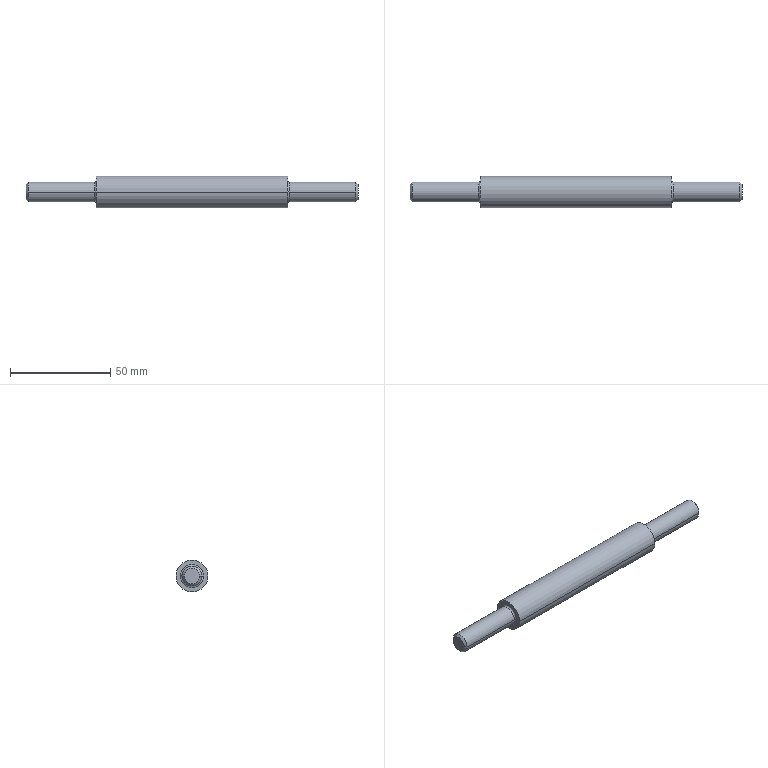Part | NX | features BREP 1 | 1 solid | 18 faces | box 165.354 x 15.875 x 15.875 mm | volume 24166 mm3 | cylinder 6 | plane 4 | torus 4 | cone 4 | commonest cylinder face diameters 9.842 x4 15.875 x2
STEP:
#1=CARTESIAN_POINT('',(-47.625,7.938,0.));
#2=VERTEX_POINT('',#1);
#3=CARTESIAN_POINT('',(-47.625,-7.938,0.));
#4=VERTEX_POINT('',#3);
#5=CARTESIAN_POINT('',(-47.625,0.,0.));
#6=DIRECTION('',(1.,0.,0.));
#7=DIRECTION('',(0.,1.,0.));
#8=AXIS2_PLACEMENT_3D('',#5,#6,#7);
#9=CIRCLE('',#8,7.938);
#10=EDGE_CURVE('',#2,#4,#9,.T.);
#11=ORIENTED_EDGE('',*,*,#10,.F.);
#12=CARTESIAN_POINT('',(-47.625,0.,0.));
#13=DIRECTION('',(1.,0.,0.));
#14=DIRECTION('',(0.,-1.,0.));
#15=AXIS2_PLACEMENT_3D('',#12,#13,#14);
#16=CIRCLE('',#15,7.938);
#17=EDGE_CURVE('',#4,#2,#16,.T.);
#18=ORIENTED_EDGE('',*,*,#17,.F.);
#19=EDGE_LOOP('',(#11,#18));
#20=FACE_BOUND('',#19,.T.);
#21=CARTESIAN_POINT('',(-47.625,5.715,0.));
#22=VERTEX_POINT('',#21);
#23=CARTESIAN_POINT('',(-47.625,-5.715,0.));
#24=VERTEX_POINT('',#23);
#25=CARTESIAN_POINT('',(-47.625,0.,0.));
#26=DIRECTION('',(-1.,0.,0.));
#27=DIRECTION('',(0.,1.,0.));
#28=AXIS2_PLACEMENT_3D('',#25,#26,#27);
#29=CIRCLE('',#28,5.715);
#30=EDGE_CURVE('',#22,#24,#29,.T.);
#31=ORIENTED_EDGE('',*,*,#30,.F.);
#32=CARTESIAN_POINT('',(-47.625,0.,0.));
#33=DIRECTION('',(-1.,0.,0.));
#34=DIRECTION('',(0.,-1.,0.));
#35=AXIS2_PLACEMENT_3D('',#32,#33,#34);
#36=CIRCLE('',#35,5.715);
#37=EDGE_CURVE('',#24,#22,#36,.T.);
#38=ORIENTED_EDGE('',*,*,#37,.F.);
#39=EDGE_LOOP('',(#31,#38));
#40=FACE_BOUND('',#39,.T.);
#41=CARTESIAN_POINT('',(-47.625,0.,0.));
#42=DIRECTION('',(1.,0.,0.));
#43=DIRECTION('',(0.,1.,0.));
#44=AXIS2_PLACEMENT_3D('',#41,#42,#43);
#45=PLANE('',#44);
#46=ADVANCED_FACE('',(#20,#40),#45,.F.);
#47=CARTESIAN_POINT('',(47.625,7.938,0.));
#48=VERTEX_POINT('',#47);
#49=CARTESIAN_POINT('',(-47.625,7.938,0.));
#50=DIRECTION('',(1.,0.,0.));
#51=VECTOR('',#50,1000.);
#52=LINE('',#49,#51);
#53=EDGE_CURVE('',#48,#2,#52,.F.);
#54=ORIENTED_EDGE('',*,*,#53,.F.);
#55=CARTESIAN_POINT('',(47.625,-7.938,0.));
#56=VERTEX_POINT('',#55);
#57=CARTESIAN_POINT('',(47.625,0.,0.));
#58=DIRECTION('',(1.,0.,0.));
#59=DIRECTION('',(0.,-1.,0.));
#60=AXIS2_PLACEMENT_3D('',#57,#58,#59);
#61=CIRCLE('',#60,7.938);
#62=EDGE_CURVE('',#56,#48,#61,.T.);
#63=ORIENTED_EDGE('',*,*,#62,.F.);
#64=CARTESIAN_POINT('',(-47.625,-7.938,0.));
#65=DIRECTION('',(1.,0.,0.));
#66=VECTOR('',#65,1000.);
#67=LINE('',#64,#66);
#68=EDGE_CURVE('',#56,#4,#67,.F.);
#69=ORIENTED_EDGE('',*,*,#68,.T.);
#70=ORIENTED_EDGE('',*,*,#17,.T.);
#71=EDGE_LOOP('',(#54,#63,#69,#70));
#72=FACE_BOUND('',#71,.T.);
#73=CARTESIAN_POINT('',(-47.625,0.,0.));
#74=DIRECTION('',(1.,0.,0.));
#75=DIRECTION('',(0.,-1.,0.));
#76=AXIS2_PLACEMENT_3D('',#73,#74,#75);
#77=CYLINDRICAL_SURFACE('',#76,7.938);
#78=ADVANCED_FACE('',(#72),#77,.T.);
#79=ORIENTED_EDGE('',*,*,#68,.F.);
#80=CARTESIAN_POINT('',(47.625,0.,0.));
#81=DIRECTION('',(1.,0.,0.));
#82=DIRECTION('',(0.,1.,0.));
#83=AXIS2_PLACEMENT_3D('',#80,#81,#82);
#84=CIRCLE('',#83,7.938);
#85=EDGE_CURVE('',#48,#56,#84,.T.);
#86=ORIENTED_EDGE('',*,*,#85,.F.);
#87=ORIENTED_EDGE('',*,*,#53,.T.);
#88=ORIENTED_EDGE('',*,*,#10,.T.);
#89=EDGE_LOOP('',(#79,#86,#87,#88));
#90=FACE_BOUND('',#89,.T.);
#91=CARTESIAN_POINT('',(-47.625,0.,0.));
#92=DIRECTION('',(1.,0.,0.));
#93=DIRECTION('',(0.,-1.,0.));
#94=AXIS2_PLACEMENT_3D('',#91,#92,#93);
#95=CYLINDRICAL_SURFACE('',#94,7.938);
#96=ADVANCED_FACE('',(#90),#95,.T.);
#97=ORIENTED_EDGE('',*,*,#85,.T.);
#98=ORIENTED_EDGE('',*,*,#62,.T.);
#99=EDGE_LOOP('',(#97,#98));
#100=FACE_BOUND('',#99,.T.);
#101=CARTESIAN_POINT('',(47.625,-5.715,0.));
#102=VERTEX_POINT('',#101);
#103=CARTESIAN_POINT('',(47.625,5.715,0.));
#104=VERTEX_POINT('',#103);
#105=CARTESIAN_POINT('',(47.625,0.,0.));
#106=DIRECTION('',(1.,0.,0.));
#107=DIRECTION('',(0.,-1.,0.));
#108=AXIS2_PLACEMENT_3D('',#105,#106,#107);
#109=CIRCLE('',#108,5.715);
#110=EDGE_CURVE('',#102,#104,#109,.T.);
#111=ORIENTED_EDGE('',*,*,#110,.F.);
#112=CARTESIAN_POINT('',(47.625,0.,0.));
#113=DIRECTION('',(1.,0.,0.));
#114=DIRECTION('',(0.,1.,0.));
#115=AXIS2_PLACEMENT_3D('',#112,#113,#114);
#116=CIRCLE('',#115,5.715);
#117=EDGE_CURVE('',#104,#102,#116,.T.);
#118=ORIENTED_EDGE('',*,*,#117,.F.);
#119=EDGE_LOOP('',(#111,#118));
#120=FACE_BOUND('',#119,.T.);
#121=CARTESIAN_POINT('',(47.625,0.,0.));
#122=DIRECTION('',(1.,0.,0.));
#123=DIRECTION('',(0.,1.,0.));
#124=AXIS2_PLACEMENT_3D('',#121,#122,#123);
#125=PLANE('',#124);
#126=ADVANCED_FACE('',(#100,#120),#125,.T.);
#127=CARTESIAN_POINT('',(48.419,-4.921,0.));
#128=VERTEX_POINT('',#127);
#129=CARTESIAN_POINT('',(48.419,-5.715,0.000000001));
#130=DIRECTION('',(0.,0.,-1.));
#131=DIRECTION('',(-1.,0.000000001,0.));
#132=AXIS2_PLACEMENT_3D('',#129,#130,#131);
#133=CIRCLE('',#132,0.7938);
#134=EDGE_CURVE('',#102,#128,#133,.T.);
#135=ORIENTED_EDGE('',*,*,#134,.T.);
#136=CARTESIAN_POINT('',(48.419,4.921,0.));
#137=VERTEX_POINT('',#136);
#138=CARTESIAN_POINT('',(48.419,0.,0.));
#139=DIRECTION('',(1.,0.,0.));
#140=DIRECTION('',(0.,1.,0.));
#141=AXIS2_PLACEMENT_3D('',#138,#139,#140);
#142=CIRCLE('',#141,4.921);
#143=EDGE_CURVE('',#137,#128,#142,.T.);
#144=ORIENTED_EDGE('',*,*,#143,.F.);
#145=CARTESIAN_POINT('',(48.419,5.715,-0.000000001));
#146=DIRECTION('',(0.,0.,1.));
#147=DIRECTION('',(-1.,-0.000000001,0.));
#148=AXIS2_PLACEMENT_3D('',#145,#146,#147);
#149=CIRCLE('',#148,0.7938);
#150=EDGE_CURVE('',#104,#137,#149,.T.);
#151=ORIENTED_EDGE('',*,*,#150,.F.);
#152=ORIENTED_EDGE('',*,*,#117,.T.);
#153=EDGE_LOOP('',(#135,#144,#151,#152));
#154=FACE_BOUND('',#153,.T.);
#155=CARTESIAN_POINT('',(48.419,0.,0.));
#156=DIRECTION('',(1.,0.,0.));
#157=DIRECTION('',(0.,0.9986,-0.05211));
#158=AXIS2_PLACEMENT_3D('',#155,#156,#157);
#159=TOROIDAL_SURFACE('',#158,5.715,0.7937);
#160=ADVANCED_FACE('',(#154),#159,.F.);
#161=ORIENTED_EDGE('',*,*,#150,.T.);
#162=CARTESIAN_POINT('',(48.419,0.,0.));
#163=DIRECTION('',(1.,0.,0.));
#164=DIRECTION('',(0.,-1.,0.));
#165=AXIS2_PLACEMENT_3D('',#162,#163,#164);
#166=CIRCLE('',#165,4.921);
#167=EDGE_CURVE('',#128,#137,#166,.T.);
#168=ORIENTED_EDGE('',*,*,#167,.F.);
#169=ORIENTED_EDGE('',*,*,#134,.F.);
#170=ORIENTED_EDGE('',*,*,#110,.T.);
#171=EDGE_LOOP('',(#161,#168,#169,#170));
#172=FACE_BOUND('',#171,.T.);
#173=CARTESIAN_POINT('',(48.419,0.,0.));
#174=DIRECTION('',(1.,0.,0.));
#175=DIRECTION('',(0.,-0.9986,0.05211));
#176=AXIS2_PLACEMENT_3D('',#173,#174,#175);
#177=TOROIDAL_SURFACE('',#176,5.715,0.7937);
#178=ADVANCED_FACE('',(#172),#177,.F.);
#179=CARTESIAN_POINT('',(81.661,4.921,0.));
#180=VERTEX_POINT('',#179);
#181=CARTESIAN_POINT('',(48.419,4.921,0.000000001));
#182=DIRECTION('',(1.,0.,0.));
#183=VECTOR('',#182,1000.);
#184=LINE('',#181,#183);
#185=EDGE_CURVE('',#180,#137,#184,.F.);
#186=ORIENTED_EDGE('',*,*,#185,.F.);
#187=CARTESIAN_POINT('',(81.661,-4.921,0.));
#188=VERTEX_POINT('',#187);
#189=CARTESIAN_POINT('',(81.661,0.,0.));
#190=DIRECTION('',(1.,0.,0.));
#191=DIRECTION('',(0.,-1.,0.));
#192=AXIS2_PLACEMENT_3D('',#189,#190,#191);
#193=CIRCLE('',#192,4.921);
#194=EDGE_CURVE('',#188,#180,#193,.T.);
#195=ORIENTED_EDGE('',*,*,#194,.F.);
#196=CARTESIAN_POINT('',(48.419,-4.921,-0.000000001));
#197=DIRECTION('',(1.,0.,0.));
#198=VECTOR('',#197,1000.);
#199=LINE('',#196,#198);
#200=EDGE_CURVE('',#188,#128,#199,.F.);
#201=ORIENTED_EDGE('',*,*,#200,.T.);
#202=ORIENTED_EDGE('',*,*,#167,.T.);
#203=EDGE_LOOP('',(#186,#195,#201,#202));
#204=FACE_BOUND('',#203,.T.);
#205=CARTESIAN_POINT('',(47.625,0.,0.));
#206=DIRECTION('',(1.,0.,0.));
#207=DIRECTION('',(0.,-1.,0.));
#208=AXIS2_PLACEMENT_3D('',#205,#206,#207);
#209=CYLINDRICAL_SURFACE('',#208,4.921);
#210=ADVANCED_FACE('',(#204),#209,.T.);
#211=ORIENTED_EDGE('',*,*,#200,.F.);
#212=CARTESIAN_POINT('',(81.661,0.,0.));
#213=DIRECTION('',(1.,0.,0.));
#214=DIRECTION('',(0.,1.,0.));
#215=AXIS2_PLACEMENT_3D('',#212,#213,#214);
#216=CIRCLE('',#215,4.921);
#217=EDGE_CURVE('',#180,#188,#216,.T.);
#218=ORIENTED_EDGE('',*,*,#217,.F.);
#219=ORIENTED_EDGE('',*,*,#185,.T.);
#220=ORIENTED_EDGE('',*,*,#143,.T.);
#221=EDGE_LOOP('',(#211,#218,#219,#220));
#222=FACE_BOUND('',#221,.T.);
#223=CARTESIAN_POINT('',(47.625,0.,0.));
#224=DIRECTION('',(1.,0.,0.));
#225=DIRECTION('',(0.,-1.,0.));
#226=AXIS2_PLACEMENT_3D('',#223,#224,#225);
#227=CYLINDRICAL_SURFACE('',#226,4.921);
#228=ADVANCED_FACE('',(#222),#227,.T.);
#229=CARTESIAN_POINT('',(82.677,3.905,0.));
#230=VERTEX_POINT('',#229);
#231=CARTESIAN_POINT('',(82.677,3.905,0.));
#232=DIRECTION('',(-0.7071,0.7071,0.));
#233=VECTOR('',#232,1000.);
#234=LINE('',#231,#233);
#235=EDGE_CURVE('',#180,#230,#234,.F.);
#236=ORIENTED_EDGE('',*,*,#235,.F.);
#237=ORIENTED_EDGE('',*,*,#217,.T.);
#238=CARTESIAN_POINT('',(82.677,-3.905,0.));
#239=VERTEX_POINT('',#238);
#240=CARTESIAN_POINT('',(82.677,-3.905,0.));
#241=DIRECTION('',(-0.7071,-0.7071,0.));
#242=VECTOR('',#241,1000.);
#243=LINE('',#240,#242);
#244=EDGE_CURVE('',#188,#239,#243,.F.);
#245=ORIENTED_EDGE('',*,*,#244,.T.);
#246=CARTESIAN_POINT('',(82.677,0.,0.));
#247=DIRECTION('',(1.,0.,0.));
#248=DIRECTION('',(0.,1.,0.));
#249=AXIS2_PLACEMENT_3D('',#246,#247,#248);
#250=CIRCLE('',#249,3.905);
#251=EDGE_CURVE('',#230,#239,#250,.T.);
#252=ORIENTED_EDGE('',*,*,#251,.F.);
#253=EDGE_LOOP('',(#236,#237,#245,#252));
#254=FACE_BOUND('',#253,.T.);
#255=CARTESIAN_POINT('',(82.169,0.,0.));
#256=DIRECTION('',(-1.,0.,0.));
#257=DIRECTION('',(0.,1.,0.));
#258=AXIS2_PLACEMENT_3D('',#255,#256,#257);
#259=CONICAL_SURFACE('',#258,4.413,0.7854);
#260=ADVANCED_FACE('',(#254),#259,.T.);
#261=ORIENTED_EDGE('',*,*,#251,.T.);
#262=CARTESIAN_POINT('',(82.677,0.,0.));
#263=DIRECTION('',(1.,0.,0.));
#264=DIRECTION('',(0.,-1.,0.));
#265=AXIS2_PLACEMENT_3D('',#262,#263,#264);
#266=CIRCLE('',#265,3.905);
#267=EDGE_CURVE('',#239,#230,#266,.T.);
#268=ORIENTED_EDGE('',*,*,#267,.T.);
#269=EDGE_LOOP('',(#261,#268));
#270=FACE_BOUND('',#269,.T.);
#271=CARTESIAN_POINT('',(82.677,0.,0.));
#272=DIRECTION('',(1.,0.,0.));
#273=DIRECTION('',(0.,1.,0.));
#274=AXIS2_PLACEMENT_3D('',#271,#272,#273);
#275=PLANE('',#274);
#276=ADVANCED_FACE('',(#270),#275,.T.);
#277=ORIENTED_EDGE('',*,*,#244,.F.);
#278=ORIENTED_EDGE('',*,*,#194,.T.);
#279=ORIENTED_EDGE('',*,*,#235,.T.);
#280=ORIENTED_EDGE('',*,*,#267,.F.);
#281=EDGE_LOOP('',(#277,#278,#279,#280));
#282=FACE_BOUND('',#281,.T.);
#283=CARTESIAN_POINT('',(82.169,0.,0.));
#284=DIRECTION('',(-1.,0.,0.));
#285=DIRECTION('',(0.,1.,0.));
#286=AXIS2_PLACEMENT_3D('',#283,#284,#285);
#287=CONICAL_SURFACE('',#286,4.413,0.7854);
#288=ADVANCED_FACE('',(#282),#287,.T.);
#289=CARTESIAN_POINT('',(-48.419,4.921,0.));
#290=VERTEX_POINT('',#289);
#291=CARTESIAN_POINT('',(-48.419,5.715,0.000000001));
#292=DIRECTION('',(0.,0.,-1.));
#293=DIRECTION('',(1.,-0.000000001,0.));
#294=AXIS2_PLACEMENT_3D('',#291,#292,#293);
#295=CIRCLE('',#294,0.7938);
#296=EDGE_CURVE('',#290,#22,#295,.F.);
#297=ORIENTED_EDGE('',*,*,#296,.F.);
#298=CARTESIAN_POINT('',(-48.419,-4.921,0.));
#299=VERTEX_POINT('',#298);
#300=CARTESIAN_POINT('',(-48.419,0.,0.));
#301=DIRECTION('',(-1.,0.,0.));
#302=DIRECTION('',(0.,-1.,0.));
#303=AXIS2_PLACEMENT_3D('',#300,#301,#302);
#304=CIRCLE('',#303,4.921);
#305=EDGE_CURVE('',#299,#290,#304,.T.);
#306=ORIENTED_EDGE('',*,*,#305,.F.);
#307=CARTESIAN_POINT('',(-48.419,-5.715,-0.000000001));
#308=DIRECTION('',(0.,0.,1.));
#309=DIRECTION('',(1.,0.000000001,0.));
#310=AXIS2_PLACEMENT_3D('',#307,#308,#309);
#311=CIRCLE('',#310,0.7938);
#312=EDGE_CURVE('',#299,#24,#311,.F.);
#313=ORIENTED_EDGE('',*,*,#312,.T.);
#314=ORIENTED_EDGE('',*,*,#37,.T.);
#315=EDGE_LOOP('',(#297,#306,#313,#314));
#316=FACE_BOUND('',#315,.T.);
#317=CARTESIAN_POINT('',(-48.419,0.,0.));
#318=DIRECTION('',(-1.,0.,0.));
#319=DIRECTION('',(0.,-0.9986,-0.05211));
#320=AXIS2_PLACEMENT_3D('',#317,#318,#319);
#321=TOROIDAL_SURFACE('',#320,5.715,0.7937);
#322=ADVANCED_FACE('',(#316),#321,.F.);
#323=ORIENTED_EDGE('',*,*,#312,.F.);
#324=CARTESIAN_POINT('',(-48.419,0.,0.));
#325=DIRECTION('',(-1.,0.,0.));
#326=DIRECTION('',(0.,1.,0.));
#327=AXIS2_PLACEMENT_3D('',#324,#325,#326);
#328=CIRCLE('',#327,4.921);
#329=EDGE_CURVE('',#290,#299,#328,.T.);
#330=ORIENTED_EDGE('',*,*,#329,.F.);
#331=ORIENTED_EDGE('',*,*,#296,.T.);
#332=ORIENTED_EDGE('',*,*,#30,.T.);
#333=EDGE_LOOP('',(#323,#330,#331,#332));
#334=FACE_BOUND('',#333,.T.);
#335=CARTESIAN_POINT('',(-48.419,0.,0.));
#336=DIRECTION('',(-1.,0.,0.));
#337=DIRECTION('',(0.,0.9986,0.05211));
#338=AXIS2_PLACEMENT_3D('',#335,#336,#337);
#339=TOROIDAL_SURFACE('',#338,5.715,0.7937);
#340=ADVANCED_FACE('',(#334),#339,.F.);
#341=CARTESIAN_POINT('',(-81.661,-4.921,0.));
#342=VERTEX_POINT('',#341);
#343=CARTESIAN_POINT('',(-48.419,-4.921,0.000000001));
#344=DIRECTION('',(-1.,0.,0.));
#345=VECTOR('',#344,1000.);
#346=LINE('',#343,#345);
#347=EDGE_CURVE('',#299,#342,#346,.T.);
#348=ORIENTED_EDGE('',*,*,#347,.T.);
#349=CARTESIAN_POINT('',(-81.661,4.921,0.));
#350=VERTEX_POINT('',#349);
#351=CARTESIAN_POINT('',(-81.661,0.,0.));
#352=DIRECTION('',(-1.,0.,0.));
#353=DIRECTION('',(0.,1.,0.));
#354=AXIS2_PLACEMENT_3D('',#351,#352,#353);
#355=CIRCLE('',#354,4.921);
#356=EDGE_CURVE('',#350,#342,#355,.T.);
#357=ORIENTED_EDGE('',*,*,#356,.F.);
#358=CARTESIAN_POINT('',(-48.419,4.921,-0.000000001));
#359=DIRECTION('',(-1.,0.,0.));
#360=VECTOR('',#359,1000.);
#361=LINE('',#358,#360);
#362=EDGE_CURVE('',#290,#350,#361,.T.);
#363=ORIENTED_EDGE('',*,*,#362,.F.);
#364=ORIENTED_EDGE('',*,*,#329,.T.);
#365=EDGE_LOOP('',(#348,#357,#363,#364));
#366=FACE_BOUND('',#365,.T.);
#367=CARTESIAN_POINT('',(-47.625,0.,0.));
#368=DIRECTION('',(-1.,0.,0.));
#369=DIRECTION('',(0.,1.,0.));
#370=AXIS2_PLACEMENT_3D('',#367,#368,#369);
#371=CYLINDRICAL_SURFACE('',#370,4.921);
#372=ADVANCED_FACE('',(#366),#371,.T.);
#373=ORIENTED_EDGE('',*,*,#362,.T.);
#374=CARTESIAN_POINT('',(-81.661,0.,0.));
#375=DIRECTION('',(-1.,0.,0.));
#376=DIRECTION('',(0.,-1.,0.));
#377=AXIS2_PLACEMENT_3D('',#374,#375,#376);
#378=CIRCLE('',#377,4.921);
#379=EDGE_CURVE('',#342,#350,#378,.T.);
#380=ORIENTED_EDGE('',*,*,#379,.F.);
#381=ORIENTED_EDGE('',*,*,#347,.F.);
#382=ORIENTED_EDGE('',*,*,#305,.T.);
#383=EDGE_LOOP('',(#373,#380,#381,#382));
#384=FACE_BOUND('',#383,.T.);
#385=CARTESIAN_POINT('',(-47.625,0.,0.));
#386=DIRECTION('',(-1.,0.,0.));
#387=DIRECTION('',(0.,1.,0.));
#388=AXIS2_PLACEMENT_3D('',#385,#386,#387);
#389=CYLINDRICAL_SURFACE('',#388,4.921);
#390=ADVANCED_FACE('',(#384),#389,.T.);
#391=CARTESIAN_POINT('',(-82.677,-3.905,0.));
#392=VERTEX_POINT('',#391);
#393=CARTESIAN_POINT('',(-82.677,-3.905,0.));
#394=DIRECTION('',(0.7071,-0.7071,0.));
#395=VECTOR('',#394,1000.);
#396=LINE('',#393,#395);
#397=EDGE_CURVE('',#392,#342,#396,.T.);
#398=ORIENTED_EDGE('',*,*,#397,.T.);
#399=ORIENTED_EDGE('',*,*,#379,.T.);
#400=CARTESIAN_POINT('',(-82.677,3.905,0.));
#401=VERTEX_POINT('',#400);
#402=CARTESIAN_POINT('',(-82.677,3.905,0.));
#403=DIRECTION('',(0.7071,0.7071,0.));
#404=VECTOR('',#403,1000.);
#405=LINE('',#402,#404);
#406=EDGE_CURVE('',#401,#350,#405,.T.);
#407=ORIENTED_EDGE('',*,*,#406,.F.);
#408=CARTESIAN_POINT('',(-82.677,0.,0.));
#409=DIRECTION('',(-1.,0.,0.));
#410=DIRECTION('',(0.,-1.,0.));
#411=AXIS2_PLACEMENT_3D('',#408,#409,#410);
#412=CIRCLE('',#411,3.905);
#413=EDGE_CURVE('',#392,#401,#412,.T.);
#414=ORIENTED_EDGE('',*,*,#413,.F.);
#415=EDGE_LOOP('',(#398,#399,#407,#414));
#416=FACE_BOUND('',#415,.T.);
#417=CARTESIAN_POINT('',(-82.169,0.,0.));
#418=DIRECTION('',(1.,0.,0.));
#419=DIRECTION('',(0.,-1.,0.));
#420=AXIS2_PLACEMENT_3D('',#417,#418,#419);
#421=CONICAL_SURFACE('',#420,4.413,0.7854);
#422=ADVANCED_FACE('',(#416),#421,.T.);
#423=ORIENTED_EDGE('',*,*,#413,.T.);
#424=CARTESIAN_POINT('',(-82.677,0.,0.));
#425=DIRECTION('',(-1.,0.,0.));
#426=DIRECTION('',(0.,1.,0.));
#427=AXIS2_PLACEMENT_3D('',#424,#425,#426);
#428=CIRCLE('',#427,3.905);
#429=EDGE_CURVE('',#401,#392,#428,.T.);
#430=ORIENTED_EDGE('',*,*,#429,.T.);
#431=EDGE_LOOP('',(#423,#430));
#432=FACE_BOUND('',#431,.T.);
#433=CARTESIAN_POINT('',(-82.677,0.,0.));
#434=DIRECTION('',(-1.,0.,0.));
#435=DIRECTION('',(0.,0.,1.));
#436=AXIS2_PLACEMENT_3D('',#433,#434,#435);
#437=PLANE('',#436);
#438=ADVANCED_FACE('',(#432),#437,.T.);
#439=ORIENTED_EDGE('',*,*,#406,.T.);
#440=ORIENTED_EDGE('',*,*,#356,.T.);
#441=ORIENTED_EDGE('',*,*,#397,.F.);
#442=ORIENTED_EDGE('',*,*,#429,.F.);
#443=EDGE_LOOP('',(#439,#440,#441,#442));
#444=FACE_BOUND('',#443,.T.);
#445=CARTESIAN_POINT('',(-82.169,0.,0.));
#446=DIRECTION('',(1.,0.,0.));
#447=DIRECTION('',(0.,-1.,0.));
#448=AXIS2_PLACEMENT_3D('',#445,#446,#447);
#449=CONICAL_SURFACE('',#448,4.413,0.7854);
#450=ADVANCED_FACE('',(#444),#449,.T.);
#451=CLOSED_SHELL('',(#46,#78,#96,#126,#160,#178,#210,#228,#260,#276,#288,#322,#340,#372,#390,#422,#438,#450));
#452=MANIFOLD_SOLID_BREP('',#451);
#453=(LENGTH_UNIT()NAMED_UNIT(*)SI_UNIT(.MILLI.,.METRE.));
#454=UNCERTAINTY_MEASURE_WITH_UNIT(LENGTH_MEASURE(0.00001),#453,'','');
#455=(NAMED_UNIT(*)PLANE_ANGLE_UNIT()SI_UNIT($,.RADIAN.));
#456=(NAMED_UNIT(*)SI_UNIT($,.STERADIAN.)SOLID_ANGLE_UNIT());
#457=(GEOMETRIC_REPRESENTATION_CONTEXT(3)GLOBAL_UNCERTAINTY_ASSIGNED_CONTEXT((#454))GLOBAL_UNIT_ASSIGNED_CONTEXT((#453,#455,#456))REPRESENTATION_CONTEXT('',''));
#458=ADVANCED_BREP_SHAPE_REPRESENTATION('',(#452),#457);